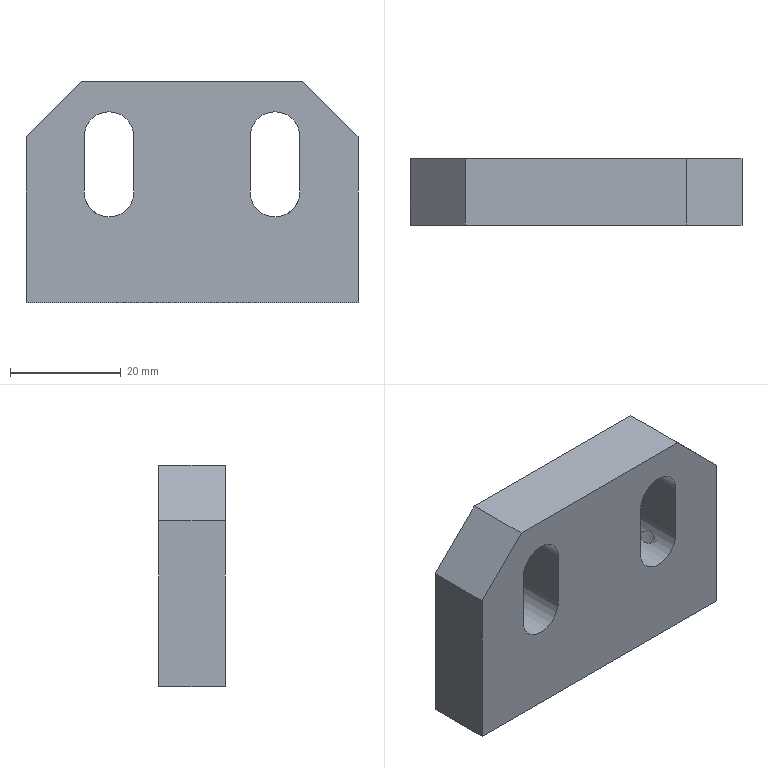Part | SolidWorks | features BaseBody 1 | 1 solid | 30 faces | box 60 x 12 x 40 mm | volume 22885 mm3 | cylinder 12 | plane 12 | cone 6 | commonest cylinder face diameters 5 x6 9 x6
STEP:
#1=CARTESIAN_POINT('',(15.,0.,14.5));
#2=VERTEX_POINT('',#1);
#3=CARTESIAN_POINT('',(19.5,0.,10.));
#4=VERTEX_POINT('',#3);
#5=CARTESIAN_POINT('',(15.,0.,10.));
#6=DIRECTION('',(0.,1.,0.));
#7=DIRECTION('',(0.,0.,-1.));
#8=AXIS2_PLACEMENT_3D('',#5,#6,#7);
#9=CIRCLE('',#8,4.5);
#10=EDGE_CURVE('',#2,#4,#9,.T.);
#11=ORIENTED_EDGE('',*,*,#10,.F.);
#12=CARTESIAN_POINT('',(15.,12.,14.5));
#13=VERTEX_POINT('',#12);
#14=CARTESIAN_POINT('',(15.,0.,14.5));
#15=DIRECTION('',(0.,1.,0.));
#16=VECTOR('',#15,1000.);
#17=LINE('',#14,#16);
#18=EDGE_CURVE('',#2,#13,#17,.T.);
#19=ORIENTED_EDGE('',*,*,#18,.T.);
#20=CARTESIAN_POINT('',(19.5,12.,10.));
#21=VERTEX_POINT('',#20);
#22=CARTESIAN_POINT('',(15.,12.,10.));
#23=DIRECTION('',(0.,1.,0.));
#24=DIRECTION('',(0.,0.,-1.));
#25=AXIS2_PLACEMENT_3D('',#22,#23,#24);
#26=CIRCLE('',#25,4.5);
#27=EDGE_CURVE('',#13,#21,#26,.T.);
#28=ORIENTED_EDGE('',*,*,#27,.T.);
#29=CARTESIAN_POINT('',(19.5,0.,10.));
#30=DIRECTION('',(0.,1.,0.));
#31=VECTOR('',#30,1000.);
#32=LINE('',#29,#31);
#33=EDGE_CURVE('',#4,#21,#32,.T.);
#34=ORIENTED_EDGE('',*,*,#33,.F.);
#35=EDGE_LOOP('',(#11,#19,#28,#34));
#36=FACE_OUTER_BOUND('',#35,.T.);
#37=CARTESIAN_POINT('',(15.,0.,10.));
#38=DIRECTION('',(0.,1.,0.));
#39=DIRECTION('',(0.,0.,1.));
#40=AXIS2_PLACEMENT_3D('',#37,#38,#39);
#41=CYLINDRICAL_SURFACE('',#40,4.5);
#42=ADVANCED_FACE('',(#36),#41,.F.);
#43=CARTESIAN_POINT('',(-15.,0.,14.5));
#44=VERTEX_POINT('',#43);
#45=CARTESIAN_POINT('',(-10.5,0.,10.));
#46=VERTEX_POINT('',#45);
#47=CARTESIAN_POINT('',(-15.,0.,10.));
#48=DIRECTION('',(0.,1.,0.));
#49=DIRECTION('',(0.,0.,1.));
#50=AXIS2_PLACEMENT_3D('',#47,#48,#49);
#51=CIRCLE('',#50,4.5);
#52=EDGE_CURVE('',#44,#46,#51,.T.);
#53=ORIENTED_EDGE('',*,*,#52,.F.);
#54=CARTESIAN_POINT('',(-15.,12.,14.5));
#55=VERTEX_POINT('',#54);
#56=CARTESIAN_POINT('',(-15.,0.,14.5));
#57=DIRECTION('',(0.,1.,0.));
#58=VECTOR('',#57,1000.);
#59=LINE('',#56,#58);
#60=EDGE_CURVE('',#44,#55,#59,.T.);
#61=ORIENTED_EDGE('',*,*,#60,.T.);
#62=CARTESIAN_POINT('',(-10.5,12.,10.));
#63=VERTEX_POINT('',#62);
#64=CARTESIAN_POINT('',(-15.,12.,10.));
#65=DIRECTION('',(0.,1.,0.));
#66=DIRECTION('',(0.,0.,1.));
#67=AXIS2_PLACEMENT_3D('',#64,#65,#66);
#68=CIRCLE('',#67,4.5);
#69=EDGE_CURVE('',#55,#63,#68,.T.);
#70=ORIENTED_EDGE('',*,*,#69,.T.);
#71=CARTESIAN_POINT('',(-10.5,0.,10.));
#72=DIRECTION('',(0.,1.,0.));
#73=VECTOR('',#72,1000.);
#74=LINE('',#71,#73);
#75=EDGE_CURVE('',#46,#63,#74,.T.);
#76=ORIENTED_EDGE('',*,*,#75,.F.);
#77=EDGE_LOOP('',(#53,#61,#70,#76));
#78=FACE_OUTER_BOUND('',#77,.T.);
#79=CARTESIAN_POINT('',(-15.,0.,10.));
#80=DIRECTION('',(0.,1.,0.));
#81=DIRECTION('',(0.,0.,1.));
#82=AXIS2_PLACEMENT_3D('',#79,#80,#81);
#83=CYLINDRICAL_SURFACE('',#82,4.5);
#84=ADVANCED_FACE('',(#78),#83,.F.);
#85=CARTESIAN_POINT('',(22.5,6.,-3.));
#86=VERTEX_POINT('',#85);
#87=CARTESIAN_POINT('',(18.354,4.118,-3.));
#88=VERTEX_POINT('',#87);
#89=CARTESIAN_POINT('',(20.,6.,-3.));
#90=DIRECTION('',(0.,0.,-1.));
#91=DIRECTION('',(-1.,0.,0.));
#92=AXIS2_PLACEMENT_3D('',#89,#90,#91);
#93=CIRCLE('',#92,2.5);
#94=EDGE_CURVE('',#86,#88,#93,.T.);
#95=ORIENTED_EDGE('',*,*,#94,.F.);
#96=CARTESIAN_POINT('',(22.5,6.,-20.));
#97=VERTEX_POINT('',#96);
#98=CARTESIAN_POINT('',(22.5,6.,-20.));
#99=DIRECTION('',(0.,0.,-1.));
#100=VECTOR('',#99,1000.);
#101=LINE('',#98,#100);
#102=EDGE_CURVE('',#86,#97,#101,.T.);
#103=ORIENTED_EDGE('',*,*,#102,.T.);
#104=CARTESIAN_POINT('',(17.5,6.,-20.));
#105=VERTEX_POINT('',#104);
#106=CARTESIAN_POINT('',(20.,6.,-20.));
#107=DIRECTION('',(0.,0.,-1.));
#108=DIRECTION('',(-1.,0.,0.));
#109=AXIS2_PLACEMENT_3D('',#106,#107,#108);
#110=CIRCLE('',#109,2.5);
#111=EDGE_CURVE('',#97,#105,#110,.T.);
#112=ORIENTED_EDGE('',*,*,#111,.T.);
#113=CARTESIAN_POINT('',(17.5,6.,-3.742));
#114=VERTEX_POINT('',#113);
#115=CARTESIAN_POINT('',(17.5,6.,-20.));
#116=DIRECTION('',(0.,0.,-1.));
#117=VECTOR('',#116,1000.);
#118=LINE('',#115,#117);
#119=EDGE_CURVE('',#114,#105,#118,.T.);
#120=ORIENTED_EDGE('',*,*,#119,.F.);
#121=CARTESIAN_POINT('',(17.5,6.,-3.742));
#122=CARTESIAN_POINT('',(17.5,5.807,-3.742));
#123=CARTESIAN_POINT('',(17.522,5.618,-3.727));
#124=CARTESIAN_POINT('',(17.608,5.247,-3.667));
#125=CARTESIAN_POINT('',(17.672,5.071,-3.622));
#126=CARTESIAN_POINT('',(17.83,4.745,-3.5));
#127=CARTESIAN_POINT('',(17.926,4.594,-3.421));
#128=CARTESIAN_POINT('',(18.131,4.331,-3.235));
#129=CARTESIAN_POINT('',(18.243,4.216,-3.125));
#130=CARTESIAN_POINT('',(18.354,4.118,-3.));
#131=B_SPLINE_CURVE_WITH_KNOTS('',3,(#121,#122,#123,#124,#125,#126,#127,#128,#129,#130),.UNSPECIFIED.,.F.,.F.,(4,2,2,2,4),(0.002293,0.002866,0.003438,0.00401,0.004583),.UNSPECIFIED.);
#132=EDGE_CURVE('',#114,#88,#131,.T.);
#133=ORIENTED_EDGE('',*,*,#132,.T.);
#134=EDGE_LOOP('',(#95,#103,#112,#120,#133));
#135=FACE_OUTER_BOUND('',#134,.T.);
#136=CARTESIAN_POINT('',(20.,6.,-20.));
#137=DIRECTION('',(0.,0.,-1.));
#138=DIRECTION('',(-1.,0.,0.));
#139=AXIS2_PLACEMENT_3D('',#136,#137,#138);
#140=CYLINDRICAL_SURFACE('',#139,2.5);
#141=ADVANCED_FACE('',(#135),#140,.F.);
#142=CARTESIAN_POINT('',(20.,6.,-1.498));
#143=VERTEX_POINT('',#142);
#144=CARTESIAN_POINT('',(18.972,6.,-2.116));
#145=VERTEX_POINT('',#144);
#146=CARTESIAN_POINT('',(17.5,6.,-3.));
#147=DIRECTION('',(-0.8572,0.,-0.515));
#148=VECTOR('',#147,1000.);
#149=LINE('',#146,#148);
#150=EDGE_CURVE('',#143,#145,#149,.T.);
#151=ORIENTED_EDGE('',*,*,#150,.F.);
#152=CARTESIAN_POINT('',(22.5,6.,-3.));
#153=DIRECTION('',(0.8572,0.,-0.515));
#154=VECTOR('',#153,1000.);
#155=LINE('',#152,#154);
#156=EDGE_CURVE('',#143,#86,#155,.T.);
#157=ORIENTED_EDGE('',*,*,#156,.T.);
#158=ORIENTED_EDGE('',*,*,#94,.T.);
#159=CARTESIAN_POINT('',(18.354,4.118,-3.));
#160=CARTESIAN_POINT('',(18.522,4.387,-2.812));
#161=CARTESIAN_POINT('',(18.659,4.672,-2.627));
#162=CARTESIAN_POINT('',(18.825,5.136,-2.373));
#163=CARTESIAN_POINT('',(18.873,5.296,-2.292));
#164=CARTESIAN_POINT('',(18.947,5.633,-2.163));
#165=CARTESIAN_POINT('',(18.972,5.814,-2.116));
#166=CARTESIAN_POINT('',(18.972,6.,-2.116));
#167=B_SPLINE_CURVE_WITH_KNOTS('',3,(#159,#160,#161,#162,#163,#164,#165,#166),.UNSPECIFIED.,.F.,.F.,(4,2,2,4),(0.0002918,0.001392,0.001943,0.002493),.UNSPECIFIED.);
#168=EDGE_CURVE('',#88,#145,#167,.T.);
#169=ORIENTED_EDGE('',*,*,#168,.T.);
#170=EDGE_LOOP('',(#151,#157,#158,#169));
#171=FACE_OUTER_BOUND('',#170,.T.);
#172=CARTESIAN_POINT('',(20.,6.,-3.));
#173=DIRECTION('',(0.,0.,-1.));
#174=DIRECTION('',(-1.,0.,0.));
#175=AXIS2_PLACEMENT_3D('',#172,#173,#174);
#176=CONICAL_SURFACE('',#175,2.5,1.03);
#177=ADVANCED_FACE('',(#171),#176,.F.);
#178=CARTESIAN_POINT('',(2.5,6.,-3.));
#179=VERTEX_POINT('',#178);
#180=CARTESIAN_POINT('',(-2.5,6.,-3.));
#181=VERTEX_POINT('',#180);
#182=CARTESIAN_POINT('',(0.,6.,-3.));
#183=DIRECTION('',(0.,0.,-1.));
#184=DIRECTION('',(-1.,0.,0.));
#185=AXIS2_PLACEMENT_3D('',#182,#183,#184);
#186=CIRCLE('',#185,2.5);
#187=EDGE_CURVE('',#179,#181,#186,.T.);
#188=ORIENTED_EDGE('',*,*,#187,.F.);
#189=CARTESIAN_POINT('',(2.5,6.,-20.));
#190=VERTEX_POINT('',#189);
#191=CARTESIAN_POINT('',(2.5,6.,-20.));
#192=DIRECTION('',(0.,0.,-1.));
#193=VECTOR('',#192,1000.);
#194=LINE('',#191,#193);
#195=EDGE_CURVE('',#179,#190,#194,.T.);
#196=ORIENTED_EDGE('',*,*,#195,.T.);
#197=CARTESIAN_POINT('',(-2.5,6.,-20.));
#198=VERTEX_POINT('',#197);
#199=CARTESIAN_POINT('',(0.,6.,-20.));
#200=DIRECTION('',(0.,0.,-1.));
#201=DIRECTION('',(-1.,0.,0.));
#202=AXIS2_PLACEMENT_3D('',#199,#200,#201);
#203=CIRCLE('',#202,2.5);
#204=EDGE_CURVE('',#190,#198,#203,.T.);
#205=ORIENTED_EDGE('',*,*,#204,.T.);
#206=CARTESIAN_POINT('',(-2.5,6.,-20.));
#207=DIRECTION('',(0.,0.,-1.));
#208=VECTOR('',#207,1000.);
#209=LINE('',#206,#208);
#210=EDGE_CURVE('',#181,#198,#209,.T.);
#211=ORIENTED_EDGE('',*,*,#210,.F.);
#212=EDGE_LOOP('',(#188,#196,#205,#211));
#213=FACE_OUTER_BOUND('',#212,.T.);
#214=CARTESIAN_POINT('',(0.,6.,-20.));
#215=DIRECTION('',(0.,0.,-1.));
#216=DIRECTION('',(-1.,0.,0.));
#217=AXIS2_PLACEMENT_3D('',#214,#215,#216);
#218=CYLINDRICAL_SURFACE('',#217,2.5);
#219=ADVANCED_FACE('',(#213),#218,.F.);
#220=CARTESIAN_POINT('',(0.,6.,-1.498));
#221=VERTEX_POINT('',#220);
#222=CARTESIAN_POINT('',(-2.5,6.,-3.));
#223=DIRECTION('',(-0.8572,0.,-0.515));
#224=VECTOR('',#223,1000.);
#225=LINE('',#222,#224);
#226=EDGE_CURVE('',#221,#181,#225,.T.);
#227=ORIENTED_EDGE('',*,*,#226,.F.);
#228=CARTESIAN_POINT('',(2.5,6.,-3.));
#229=DIRECTION('',(0.8572,0.,-0.515));
#230=VECTOR('',#229,1000.);
#231=LINE('',#228,#230);
#232=EDGE_CURVE('',#221,#179,#231,.T.);
#233=ORIENTED_EDGE('',*,*,#232,.T.);
#234=ORIENTED_EDGE('',*,*,#187,.T.);
#235=EDGE_LOOP('',(#227,#233,#234));
#236=FACE_OUTER_BOUND('',#235,.T.);
#237=CARTESIAN_POINT('',(0.,6.,-3.));
#238=DIRECTION('',(0.,0.,-1.));
#239=DIRECTION('',(-1.,0.,0.));
#240=AXIS2_PLACEMENT_3D('',#237,#238,#239);
#241=CONICAL_SURFACE('',#240,2.5,1.03);
#242=ADVANCED_FACE('',(#236),#241,.F.);
#243=CARTESIAN_POINT('',(-18.354,4.118,-3.));
#244=VERTEX_POINT('',#243);
#245=CARTESIAN_POINT('',(-17.5,6.,-3.742));
#246=VERTEX_POINT('',#245);
#247=CARTESIAN_POINT('',(-18.354,4.118,-3.));
#248=CARTESIAN_POINT('',(-18.243,4.216,-3.125));
#249=CARTESIAN_POINT('',(-18.133,4.329,-3.233));
#250=CARTESIAN_POINT('',(-17.927,4.593,-3.421));
#251=CARTESIAN_POINT('',(-17.831,4.743,-3.499));
#252=CARTESIAN_POINT('',(-17.673,5.068,-3.621));
#253=CARTESIAN_POINT('',(-17.609,5.247,-3.667));
#254=CARTESIAN_POINT('',(-17.522,5.616,-3.727));
#255=CARTESIAN_POINT('',(-17.5,5.807,-3.742));
#256=CARTESIAN_POINT('',(-17.5,6.,-3.742));
#257=B_SPLINE_CURVE_WITH_KNOTS('',3,(#247,#248,#249,#250,#251,#252,#253,#254,#255,#256),.UNSPECIFIED.,.F.,.F.,(4,2,2,2,4),(0.,0.0005733,0.001147,0.00172,0.002293),.UNSPECIFIED.);
#258=EDGE_CURVE('',#244,#246,#257,.T.);
#259=ORIENTED_EDGE('',*,*,#258,.T.);
#260=CARTESIAN_POINT('',(-17.5,6.,-20.));
#261=VERTEX_POINT('',#260);
#262=CARTESIAN_POINT('',(-17.5,6.,-20.));
#263=DIRECTION('',(0.,0.,-1.));
#264=VECTOR('',#263,1000.);
#265=LINE('',#262,#264);
#266=EDGE_CURVE('',#246,#261,#265,.T.);
#267=ORIENTED_EDGE('',*,*,#266,.T.);
#268=CARTESIAN_POINT('',(-22.5,6.,-20.));
#269=VERTEX_POINT('',#268);
#270=CARTESIAN_POINT('',(-20.,6.,-20.));
#271=DIRECTION('',(0.,0.,-1.));
#272=DIRECTION('',(-1.,0.,0.));
#273=AXIS2_PLACEMENT_3D('',#270,#271,#272);
#274=CIRCLE('',#273,2.5);
#275=EDGE_CURVE('',#261,#269,#274,.T.);
#276=ORIENTED_EDGE('',*,*,#275,.T.);
#277=CARTESIAN_POINT('',(-22.5,6.,-3.));
#278=VERTEX_POINT('',#277);
#279=CARTESIAN_POINT('',(-22.5,6.,-20.));
#280=DIRECTION('',(0.,0.,-1.));
#281=VECTOR('',#280,1000.);
#282=LINE('',#279,#281);
#283=EDGE_CURVE('',#278,#269,#282,.T.);
#284=ORIENTED_EDGE('',*,*,#283,.F.);
#285=CARTESIAN_POINT('',(-20.,6.,-3.));
#286=DIRECTION('',(0.,0.,-1.));
#287=DIRECTION('',(-1.,0.,0.));
#288=AXIS2_PLACEMENT_3D('',#285,#286,#287);
#289=CIRCLE('',#288,2.5);
#290=EDGE_CURVE('',#244,#278,#289,.T.);
#291=ORIENTED_EDGE('',*,*,#290,.F.);
#292=EDGE_LOOP('',(#259,#267,#276,#284,#291));
#293=FACE_OUTER_BOUND('',#292,.T.);
#294=CARTESIAN_POINT('',(-20.,6.,-20.));
#295=DIRECTION('',(0.,0.,-1.));
#296=DIRECTION('',(-1.,0.,0.));
#297=AXIS2_PLACEMENT_3D('',#294,#295,#296);
#298=CYLINDRICAL_SURFACE('',#297,2.5);
#299=ADVANCED_FACE('',(#293),#298,.F.);
#300=CARTESIAN_POINT('',(-20.,6.,-1.498));
#301=VERTEX_POINT('',#300);
#302=CARTESIAN_POINT('',(-22.5,6.,-3.));
#303=DIRECTION('',(-0.8572,0.,-0.515));
#304=VECTOR('',#303,1000.);
#305=LINE('',#302,#304);
#306=EDGE_CURVE('',#301,#278,#305,.T.);
#307=ORIENTED_EDGE('',*,*,#306,.F.);
#308=CARTESIAN_POINT('',(-18.972,6.,-2.116));
#309=VERTEX_POINT('',#308);
#310=CARTESIAN_POINT('',(-17.5,6.,-3.));
#311=DIRECTION('',(0.8572,0.,-0.515));
#312=VECTOR('',#311,1000.);
#313=LINE('',#310,#312);
#314=EDGE_CURVE('',#301,#309,#313,.T.);
#315=ORIENTED_EDGE('',*,*,#314,.T.);
#316=CARTESIAN_POINT('',(-18.972,6.,-2.116));
#317=CARTESIAN_POINT('',(-18.972,5.813,-2.116));
#318=CARTESIAN_POINT('',(-18.947,5.632,-2.163));
#319=CARTESIAN_POINT('',(-18.873,5.294,-2.293));
#320=CARTESIAN_POINT('',(-18.825,5.136,-2.373));
#321=CARTESIAN_POINT('',(-18.715,4.829,-2.541));
#322=CARTESIAN_POINT('',(-18.653,4.68,-2.631));
#323=CARTESIAN_POINT('',(-18.514,4.392,-2.813));
#324=CARTESIAN_POINT('',(-18.438,4.252,-2.906));
#325=CARTESIAN_POINT('',(-18.354,4.118,-3.));
#326=B_SPLINE_CURVE_WITH_KNOTS('',3,(#316,#317,#318,#319,#320,#321,#322,#323,#324,#325),.UNSPECIFIED.,.F.,.F.,(4,2,2,2,4),(0.002493,0.003044,0.003596,0.004147,0.004698),.UNSPECIFIED.);
#327=EDGE_CURVE('',#309,#244,#326,.T.);
#328=ORIENTED_EDGE('',*,*,#327,.T.);
#329=ORIENTED_EDGE('',*,*,#290,.T.);
#330=EDGE_LOOP('',(#307,#315,#328,#329));
#331=FACE_OUTER_BOUND('',#330,.T.);
#332=CARTESIAN_POINT('',(-20.,6.,-3.));
#333=DIRECTION('',(0.,0.,-1.));
#334=DIRECTION('',(-1.,0.,0.));
#335=AXIS2_PLACEMENT_3D('',#332,#333,#334);
#336=CONICAL_SURFACE('',#335,2.5,1.03);
#337=ADVANCED_FACE('',(#331),#336,.F.);
#338=CARTESIAN_POINT('',(-30.,0.,-20.));
#339=VERTEX_POINT('',#338);
#340=CARTESIAN_POINT('',(-30.,0.,10.));
#341=VERTEX_POINT('',#340);
#342=CARTESIAN_POINT('',(-30.,0.,-20.));
#343=DIRECTION('',(0.,0.,1.));
#344=VECTOR('',#343,1000.);
#345=LINE('',#342,#344);
#346=EDGE_CURVE('',#339,#341,#345,.T.);
#347=ORIENTED_EDGE('',*,*,#346,.T.);
#348=CARTESIAN_POINT('',(-30.,12.,10.));
#349=VERTEX_POINT('',#348);
#350=CARTESIAN_POINT('',(-30.,12.,10.));
#351=DIRECTION('',(0.,1.,0.));
#352=VECTOR('',#351,1000.);
#353=LINE('',#350,#352);
#354=EDGE_CURVE('',#341,#349,#353,.T.);
#355=ORIENTED_EDGE('',*,*,#354,.T.);
#356=CARTESIAN_POINT('',(-30.,12.,-20.));
#357=VERTEX_POINT('',#356);
#358=CARTESIAN_POINT('',(-30.,12.,-20.));
#359=DIRECTION('',(0.,0.,1.));
#360=VECTOR('',#359,1000.);
#361=LINE('',#358,#360);
#362=EDGE_CURVE('',#357,#349,#361,.T.);
#363=ORIENTED_EDGE('',*,*,#362,.F.);
#364=CARTESIAN_POINT('',(-30.,12.,-20.));
#365=DIRECTION('',(0.,-1.,0.));
#366=VECTOR('',#365,1000.);
#367=LINE('',#364,#366);
#368=EDGE_CURVE('',#357,#339,#367,.T.);
#369=ORIENTED_EDGE('',*,*,#368,.T.);
#370=EDGE_LOOP('',(#347,#355,#363,#369));
#371=FACE_OUTER_BOUND('',#370,.T.);
#372=CARTESIAN_POINT('',(-30.,12.,-20.));
#373=DIRECTION('',(1.,0.,0.));
#374=DIRECTION('',(0.,0.,-1.));
#375=AXIS2_PLACEMENT_3D('',#372,#373,#374);
#376=PLANE('',#375);
#377=ADVANCED_FACE('',(#371),#376,.F.);
#378=CARTESIAN_POINT('',(-20.,0.,20.));
#379=VERTEX_POINT('',#378);
#380=CARTESIAN_POINT('',(20.,0.,20.));
#381=VERTEX_POINT('',#380);
#382=CARTESIAN_POINT('',(30.,0.,20.));
#383=DIRECTION('',(1.,0.,0.));
#384=VECTOR('',#383,1000.);
#385=LINE('',#382,#384);
#386=EDGE_CURVE('',#379,#381,#385,.T.);
#387=ORIENTED_EDGE('',*,*,#386,.T.);
#388=CARTESIAN_POINT('',(20.,12.,20.));
#389=VERTEX_POINT('',#388);
#390=CARTESIAN_POINT('',(20.,12.,20.));
#391=DIRECTION('',(0.,1.,0.));
#392=VECTOR('',#391,1000.);
#393=LINE('',#390,#392);
#394=EDGE_CURVE('',#381,#389,#393,.T.);
#395=ORIENTED_EDGE('',*,*,#394,.T.);
#396=CARTESIAN_POINT('',(-20.,12.,20.));
#397=VERTEX_POINT('',#396);
#398=CARTESIAN_POINT('',(30.,12.,20.));
#399=DIRECTION('',(1.,0.,0.));
#400=VECTOR('',#399,1000.);
#401=LINE('',#398,#400);
#402=EDGE_CURVE('',#397,#389,#401,.T.);
#403=ORIENTED_EDGE('',*,*,#402,.F.);
#404=CARTESIAN_POINT('',(-20.,12.,20.));
#405=DIRECTION('',(0.,-1.,0.));
#406=VECTOR('',#405,1000.);
#407=LINE('',#404,#406);
#408=EDGE_CURVE('',#397,#379,#407,.T.);
#409=ORIENTED_EDGE('',*,*,#408,.T.);
#410=EDGE_LOOP('',(#387,#395,#403,#409));
#411=FACE_OUTER_BOUND('',#410,.T.);
#412=CARTESIAN_POINT('',(30.,12.,20.));
#413=DIRECTION('',(0.,0.,-1.));
#414=DIRECTION('',(-1.,0.,0.));
#415=AXIS2_PLACEMENT_3D('',#412,#413,#414);
#416=PLANE('',#415);
#417=ADVANCED_FACE('',(#411),#416,.F.);
#418=CARTESIAN_POINT('',(30.,12.,10.));
#419=VERTEX_POINT('',#418);
#420=CARTESIAN_POINT('',(30.,12.,-20.));
#421=VERTEX_POINT('',#420);
#422=CARTESIAN_POINT('',(30.,12.,-20.));
#423=DIRECTION('',(0.,0.,-1.));
#424=VECTOR('',#423,1000.);
#425=LINE('',#422,#424);
#426=EDGE_CURVE('',#419,#421,#425,.T.);
#427=ORIENTED_EDGE('',*,*,#426,.F.);
#428=CARTESIAN_POINT('',(30.,0.,10.));
#429=VERTEX_POINT('',#428);
#430=CARTESIAN_POINT('',(30.,12.,10.));
#431=DIRECTION('',(0.,-1.,0.));
#432=VECTOR('',#431,1000.);
#433=LINE('',#430,#432);
#434=EDGE_CURVE('',#419,#429,#433,.T.);
#435=ORIENTED_EDGE('',*,*,#434,.T.);
#436=CARTESIAN_POINT('',(30.,0.,-20.));
#437=VERTEX_POINT('',#436);
#438=CARTESIAN_POINT('',(30.,0.,-20.));
#439=DIRECTION('',(0.,0.,-1.));
#440=VECTOR('',#439,1000.);
#441=LINE('',#438,#440);
#442=EDGE_CURVE('',#429,#437,#441,.T.);
#443=ORIENTED_EDGE('',*,*,#442,.T.);
#444=CARTESIAN_POINT('',(30.,12.,-20.));
#445=DIRECTION('',(0.,-1.,0.));
#446=VECTOR('',#445,1000.);
#447=LINE('',#444,#446);
#448=EDGE_CURVE('',#421,#437,#447,.T.);
#449=ORIENTED_EDGE('',*,*,#448,.F.);
#450=EDGE_LOOP('',(#427,#435,#443,#449));
#451=FACE_OUTER_BOUND('',#450,.T.);
#452=CARTESIAN_POINT('',(30.,12.,-20.));
#453=DIRECTION('',(-1.,0.,0.));
#454=DIRECTION('',(0.,0.,1.));
#455=AXIS2_PLACEMENT_3D('',#452,#453,#454);
#456=PLANE('',#455);
#457=ADVANCED_FACE('',(#451),#456,.F.);
#458=CARTESIAN_POINT('',(20.,6.,-20.));
#459=DIRECTION('',(0.,0.,-1.));
#460=DIRECTION('',(-1.,0.,0.));
#461=AXIS2_PLACEMENT_3D('',#458,#459,#460);
#462=CIRCLE('',#461,2.5);
#463=EDGE_CURVE('',#105,#97,#462,.T.);
#464=ORIENTED_EDGE('',*,*,#463,.F.);
#465=ORIENTED_EDGE('',*,*,#111,.F.);
#466=EDGE_LOOP('',(#464,#465));
#467=FACE_BOUND('',#466,.T.);
#468=CARTESIAN_POINT('',(0.,6.,-20.));
#469=DIRECTION('',(0.,0.,-1.));
#470=DIRECTION('',(-1.,0.,0.));
#471=AXIS2_PLACEMENT_3D('',#468,#469,#470);
#472=CIRCLE('',#471,2.5);
#473=EDGE_CURVE('',#198,#190,#472,.T.);
#474=ORIENTED_EDGE('',*,*,#473,.F.);
#475=ORIENTED_EDGE('',*,*,#204,.F.);
#476=EDGE_LOOP('',(#474,#475));
#477=FACE_BOUND('',#476,.T.);
#478=CARTESIAN_POINT('',(-20.,6.,-20.));
#479=DIRECTION('',(0.,0.,-1.));
#480=DIRECTION('',(-1.,0.,0.));
#481=AXIS2_PLACEMENT_3D('',#478,#479,#480);
#482=CIRCLE('',#481,2.5);
#483=EDGE_CURVE('',#269,#261,#482,.T.);
#484=ORIENTED_EDGE('',*,*,#483,.F.);
#485=ORIENTED_EDGE('',*,*,#275,.F.);
#486=EDGE_LOOP('',(#484,#485));
#487=FACE_BOUND('',#486,.T.);
#488=CARTESIAN_POINT('',(30.,0.,-20.));
#489=DIRECTION('',(-1.,0.,0.));
#490=VECTOR('',#489,1000.);
#491=LINE('',#488,#490);
#492=EDGE_CURVE('',#437,#339,#491,.T.);
#493=ORIENTED_EDGE('',*,*,#492,.T.);
#494=ORIENTED_EDGE('',*,*,#368,.F.);
#495=CARTESIAN_POINT('',(30.,12.,-20.));
#496=DIRECTION('',(-1.,0.,0.));
#497=VECTOR('',#496,1000.);
#498=LINE('',#495,#497);
#499=EDGE_CURVE('',#421,#357,#498,.T.);
#500=ORIENTED_EDGE('',*,*,#499,.F.);
#501=ORIENTED_EDGE('',*,*,#448,.T.);
#502=EDGE_LOOP('',(#493,#494,#500,#501));
#503=FACE_OUTER_BOUND('',#502,.T.);
#504=CARTESIAN_POINT('',(30.,12.,-20.));
#505=DIRECTION('',(0.,0.,1.));
#506=DIRECTION('',(1.,0.,0.));
#507=AXIS2_PLACEMENT_3D('',#504,#505,#506);
#508=PLANE('',#507);
#509=ADVANCED_FACE('',(#467,#477,#487,#503),#508,.F.);
#510=CARTESIAN_POINT('',(10.5,12.,0.));
#511=VERTEX_POINT('',#510);
#512=CARTESIAN_POINT('',(10.5,12.,10.));
#513=VERTEX_POINT('',#512);
#514=CARTESIAN_POINT('',(10.5,12.,0.));
#515=DIRECTION('',(0.,0.,1.));
#516=VECTOR('',#515,1000.);
#517=LINE('',#514,#516);
#518=EDGE_CURVE('',#511,#513,#517,.T.);
#519=ORIENTED_EDGE('',*,*,#518,.F.);
#520=CARTESIAN_POINT('',(19.5,12.,0.));
#521=VERTEX_POINT('',#520);
#522=CARTESIAN_POINT('',(15.,12.,0.));
#523=DIRECTION('',(0.,1.,0.));
#524=DIRECTION('',(0.,0.,-1.));
#525=AXIS2_PLACEMENT_3D('',#522,#523,#524);
#526=CIRCLE('',#525,4.5);
#527=EDGE_CURVE('',#521,#511,#526,.T.);
#528=ORIENTED_EDGE('',*,*,#527,.F.);
#529=CARTESIAN_POINT('',(19.5,12.,0.));
#530=DIRECTION('',(0.,0.,-1.));
#531=VECTOR('',#530,1000.);
#532=LINE('',#529,#531);
#533=EDGE_CURVE('',#21,#521,#532,.T.);
#534=ORIENTED_EDGE('',*,*,#533,.F.);
#535=ORIENTED_EDGE('',*,*,#27,.F.);
#536=CARTESIAN_POINT('',(15.,12.,10.));
#537=DIRECTION('',(0.,1.,0.));
#538=DIRECTION('',(0.,0.,-1.));
#539=AXIS2_PLACEMENT_3D('',#536,#537,#538);
#540=CIRCLE('',#539,4.5);
#541=EDGE_CURVE('',#513,#13,#540,.T.);
#542=ORIENTED_EDGE('',*,*,#541,.F.);
#543=EDGE_LOOP('',(#519,#528,#534,#535,#542));
#544=FACE_BOUND('',#543,.T.);
#545=CARTESIAN_POINT('',(-19.5,12.,0.));
#546=VERTEX_POINT('',#545);
#547=CARTESIAN_POINT('',(-19.5,12.,10.));
#548=VERTEX_POINT('',#547);
#549=CARTESIAN_POINT('',(-19.5,12.,0.));
#550=DIRECTION('',(0.,0.,1.));
#551=VECTOR('',#550,1000.);
#552=LINE('',#549,#551);
#553=EDGE_CURVE('',#546,#548,#552,.T.);
#554=ORIENTED_EDGE('',*,*,#553,.F.);
#555=CARTESIAN_POINT('',(-10.5,12.,0.));
#556=VERTEX_POINT('',#555);
#557=CARTESIAN_POINT('',(-15.,12.,0.));
#558=DIRECTION('',(0.,1.,0.));
#559=DIRECTION('',(0.,0.,1.));
#560=AXIS2_PLACEMENT_3D('',#557,#558,#559);
#561=CIRCLE('',#560,4.5);
#562=EDGE_CURVE('',#556,#546,#561,.T.);
#563=ORIENTED_EDGE('',*,*,#562,.F.);
#564=CARTESIAN_POINT('',(-10.5,12.,0.));
#565=DIRECTION('',(0.,0.,-1.));
#566=VECTOR('',#565,1000.);
#567=LINE('',#564,#566);
#568=EDGE_CURVE('',#63,#556,#567,.T.);
#569=ORIENTED_EDGE('',*,*,#568,.F.);
#570=ORIENTED_EDGE('',*,*,#69,.F.);
#571=CARTESIAN_POINT('',(-15.,12.,10.));
#572=DIRECTION('',(0.,1.,0.));
#573=DIRECTION('',(0.,0.,1.));
#574=AXIS2_PLACEMENT_3D('',#571,#572,#573);
#575=CIRCLE('',#574,4.5);
#576=EDGE_CURVE('',#548,#55,#575,.T.);
#577=ORIENTED_EDGE('',*,*,#576,.F.);
#578=EDGE_LOOP('',(#554,#563,#569,#570,#577));
#579=FACE_BOUND('',#578,.T.);
#580=ORIENTED_EDGE('',*,*,#402,.T.);
#581=CARTESIAN_POINT('',(30.,12.,10.));
#582=DIRECTION('',(0.7071,0.,-0.7071));
#583=VECTOR('',#582,1000.);
#584=LINE('',#581,#583);
#585=EDGE_CURVE('',#389,#419,#584,.T.);
#586=ORIENTED_EDGE('',*,*,#585,.T.);
#587=ORIENTED_EDGE('',*,*,#426,.T.);
#588=ORIENTED_EDGE('',*,*,#499,.T.);
#589=ORIENTED_EDGE('',*,*,#362,.T.);
#590=CARTESIAN_POINT('',(-20.,12.,20.));
#591=DIRECTION('',(0.7071,0.,0.7071));
#592=VECTOR('',#591,1000.);
#593=LINE('',#590,#592);
#594=EDGE_CURVE('',#349,#397,#593,.T.);
#595=ORIENTED_EDGE('',*,*,#594,.T.);
#596=EDGE_LOOP('',(#580,#586,#587,#588,#589,#595));
#597=FACE_OUTER_BOUND('',#596,.T.);
#598=CARTESIAN_POINT('',(0.,12.,0.));
#599=DIRECTION('',(0.,-1.,0.));
#600=DIRECTION('',(0.,0.,-1.));
#601=AXIS2_PLACEMENT_3D('',#598,#599,#600);
#602=PLANE('',#601);
#603=ADVANCED_FACE('',(#544,#579,#597),#602,.F.);
#604=CARTESIAN_POINT('',(19.5,0.,0.));
#605=VERTEX_POINT('',#604);
#606=CARTESIAN_POINT('',(10.5,0.,0.));
#607=VERTEX_POINT('',#606);
#608=CARTESIAN_POINT('',(15.,0.,0.));
#609=DIRECTION('',(0.,1.,0.));
#610=DIRECTION('',(0.,0.,-1.));
#611=AXIS2_PLACEMENT_3D('',#608,#609,#610);
#612=CIRCLE('',#611,4.5);
#613=EDGE_CURVE('',#605,#607,#612,.T.);
#614=ORIENTED_EDGE('',*,*,#613,.T.);
#615=CARTESIAN_POINT('',(10.5,0.,10.));
#616=VERTEX_POINT('',#615);
#617=CARTESIAN_POINT('',(10.5,0.,0.));
#618=DIRECTION('',(0.,0.,1.));
#619=VECTOR('',#618,1000.);
#620=LINE('',#617,#619);
#621=EDGE_CURVE('',#607,#616,#620,.T.);
#622=ORIENTED_EDGE('',*,*,#621,.T.);
#623=CARTESIAN_POINT('',(15.,0.,10.));
#624=DIRECTION('',(0.,1.,0.));
#625=DIRECTION('',(0.,0.,-1.));
#626=AXIS2_PLACEMENT_3D('',#623,#624,#625);
#627=CIRCLE('',#626,4.5);
#628=EDGE_CURVE('',#616,#2,#627,.T.);
#629=ORIENTED_EDGE('',*,*,#628,.T.);
#630=ORIENTED_EDGE('',*,*,#10,.T.);
#631=CARTESIAN_POINT('',(19.5,0.,0.));
#632=DIRECTION('',(0.,0.,-1.));
#633=VECTOR('',#632,1000.);
#634=LINE('',#631,#633);
#635=EDGE_CURVE('',#4,#605,#634,.T.);
#636=ORIENTED_EDGE('',*,*,#635,.T.);
#637=EDGE_LOOP('',(#614,#622,#629,#630,#636));
#638=FACE_BOUND('',#637,.T.);
#639=CARTESIAN_POINT('',(-10.5,0.,0.));
#640=VERTEX_POINT('',#639);
#641=CARTESIAN_POINT('',(-19.5,0.,0.));
#642=VERTEX_POINT('',#641);
#643=CARTESIAN_POINT('',(-15.,0.,0.));
#644=DIRECTION('',(0.,1.,0.));
#645=DIRECTION('',(0.,0.,1.));
#646=AXIS2_PLACEMENT_3D('',#643,#644,#645);
#647=CIRCLE('',#646,4.5);
#648=EDGE_CURVE('',#640,#642,#647,.T.);
#649=ORIENTED_EDGE('',*,*,#648,.T.);
#650=CARTESIAN_POINT('',(-19.5,0.,10.));
#651=VERTEX_POINT('',#650);
#652=CARTESIAN_POINT('',(-19.5,0.,0.));
#653=DIRECTION('',(0.,0.,1.));
#654=VECTOR('',#653,1000.);
#655=LINE('',#652,#654);
#656=EDGE_CURVE('',#642,#651,#655,.T.);
#657=ORIENTED_EDGE('',*,*,#656,.T.);
#658=CARTESIAN_POINT('',(-15.,0.,10.));
#659=DIRECTION('',(0.,1.,0.));
#660=DIRECTION('',(0.,0.,1.));
#661=AXIS2_PLACEMENT_3D('',#658,#659,#660);
#662=CIRCLE('',#661,4.5);
#663=EDGE_CURVE('',#651,#44,#662,.T.);
#664=ORIENTED_EDGE('',*,*,#663,.T.);
#665=ORIENTED_EDGE('',*,*,#52,.T.);
#666=CARTESIAN_POINT('',(-10.5,0.,0.));
#667=DIRECTION('',(0.,0.,-1.));
#668=VECTOR('',#667,1000.);
#669=LINE('',#666,#668);
#670=EDGE_CURVE('',#46,#640,#669,.T.);
#671=ORIENTED_EDGE('',*,*,#670,.T.);
#672=EDGE_LOOP('',(#649,#657,#664,#665,#671));
#673=FACE_BOUND('',#672,.T.);
#674=ORIENTED_EDGE('',*,*,#442,.F.);
#675=CARTESIAN_POINT('',(20.,0.,20.));
#676=DIRECTION('',(-0.7071,0.,0.7071));
#677=VECTOR('',#676,1000.);
#678=LINE('',#675,#677);
#679=EDGE_CURVE('',#429,#381,#678,.T.);
#680=ORIENTED_EDGE('',*,*,#679,.T.);
#681=ORIENTED_EDGE('',*,*,#386,.F.);
#682=CARTESIAN_POINT('',(-20.,0.,20.));
#683=DIRECTION('',(-0.7071,0.,-0.7071));
#684=VECTOR('',#683,1000.);
#685=LINE('',#682,#684);
#686=EDGE_CURVE('',#379,#341,#685,.T.);
#687=ORIENTED_EDGE('',*,*,#686,.T.);
#688=ORIENTED_EDGE('',*,*,#346,.F.);
#689=ORIENTED_EDGE('',*,*,#492,.F.);
#690=EDGE_LOOP('',(#674,#680,#681,#687,#688,#689));
#691=FACE_OUTER_BOUND('',#690,.T.);
#692=CARTESIAN_POINT('',(0.,0.,0.));
#693=DIRECTION('',(0.,-1.,0.));
#694=DIRECTION('',(0.,0.,-1.));
#695=AXIS2_PLACEMENT_3D('',#692,#693,#694);
#696=PLANE('',#695);
#697=ADVANCED_FACE('',(#638,#673,#691),#696,.T.);
#698=ORIENTED_EDGE('',*,*,#314,.F.);
#699=ORIENTED_EDGE('',*,*,#306,.T.);
#700=CARTESIAN_POINT('',(-18.354,7.882,-3.));
#701=VERTEX_POINT('',#700);
#702=CARTESIAN_POINT('',(-20.,6.,-3.));
#703=DIRECTION('',(0.,0.,-1.));
#704=DIRECTION('',(-1.,0.,0.));
#705=AXIS2_PLACEMENT_3D('',#702,#703,#704);
#706=CIRCLE('',#705,2.5);
#707=EDGE_CURVE('',#278,#701,#706,.T.);
#708=ORIENTED_EDGE('',*,*,#707,.T.);
#709=CARTESIAN_POINT('',(-18.354,7.882,-3.));
#710=CARTESIAN_POINT('',(-18.522,7.613,-2.812));
#711=CARTESIAN_POINT('',(-18.659,7.328,-2.627));
#712=CARTESIAN_POINT('',(-18.825,6.864,-2.373));
#713=CARTESIAN_POINT('',(-18.873,6.704,-2.292));
#714=CARTESIAN_POINT('',(-18.947,6.367,-2.163));
#715=CARTESIAN_POINT('',(-18.972,6.186,-2.116));
#716=CARTESIAN_POINT('',(-18.972,6.,-2.116));
#717=B_SPLINE_CURVE_WITH_KNOTS('',3,(#709,#710,#711,#712,#713,#714,#715,#716),.UNSPECIFIED.,.F.,.F.,(4,2,2,4),(0.0002918,0.001392,0.001943,0.002493),.UNSPECIFIED.);
#718=EDGE_CURVE('',#701,#309,#717,.T.);
#719=ORIENTED_EDGE('',*,*,#718,.T.);
#720=EDGE_LOOP('',(#698,#699,#708,#719));
#721=FACE_OUTER_BOUND('',#720,.T.);
#722=CARTESIAN_POINT('',(-20.,6.,-3.));
#723=DIRECTION('',(0.,0.,-1.));
#724=DIRECTION('',(-1.,0.,0.));
#725=AXIS2_PLACEMENT_3D('',#722,#723,#724);
#726=CONICAL_SURFACE('',#725,2.5,1.03);
#727=ADVANCED_FACE('',(#721),#726,.F.);
#728=ORIENTED_EDGE('',*,*,#266,.F.);
#729=CARTESIAN_POINT('',(-17.5,6.,-3.742));
#730=CARTESIAN_POINT('',(-17.5,6.193,-3.742));
#731=CARTESIAN_POINT('',(-17.522,6.382,-3.727));
#732=CARTESIAN_POINT('',(-17.608,6.753,-3.667));
#733=CARTESIAN_POINT('',(-17.672,6.929,-3.622));
#734=CARTESIAN_POINT('',(-17.83,7.255,-3.5));
#735=CARTESIAN_POINT('',(-17.926,7.406,-3.421));
#736=CARTESIAN_POINT('',(-18.131,7.669,-3.235));
#737=CARTESIAN_POINT('',(-18.243,7.784,-3.125));
#738=CARTESIAN_POINT('',(-18.354,7.882,-3.));
#739=B_SPLINE_CURVE_WITH_KNOTS('',3,(#729,#730,#731,#732,#733,#734,#735,#736,#737,#738),.UNSPECIFIED.,.F.,.F.,(4,2,2,2,4),(0.002293,0.002866,0.003438,0.00401,0.004583),.UNSPECIFIED.);
#740=EDGE_CURVE('',#246,#701,#739,.T.);
#741=ORIENTED_EDGE('',*,*,#740,.T.);
#742=ORIENTED_EDGE('',*,*,#707,.F.);
#743=ORIENTED_EDGE('',*,*,#283,.T.);
#744=ORIENTED_EDGE('',*,*,#483,.T.);
#745=EDGE_LOOP('',(#728,#741,#742,#743,#744));
#746=FACE_OUTER_BOUND('',#745,.T.);
#747=CARTESIAN_POINT('',(-20.,6.,-20.));
#748=DIRECTION('',(0.,0.,-1.));
#749=DIRECTION('',(-1.,0.,0.));
#750=AXIS2_PLACEMENT_3D('',#747,#748,#749);
#751=CYLINDRICAL_SURFACE('',#750,2.5);
#752=ADVANCED_FACE('',(#746),#751,.F.);
#753=ORIENTED_EDGE('',*,*,#232,.F.);
#754=ORIENTED_EDGE('',*,*,#226,.T.);
#755=CARTESIAN_POINT('',(0.,6.,-3.));
#756=DIRECTION('',(0.,0.,-1.));
#757=DIRECTION('',(-1.,0.,0.));
#758=AXIS2_PLACEMENT_3D('',#755,#756,#757);
#759=CIRCLE('',#758,2.5);
#760=EDGE_CURVE('',#181,#179,#759,.T.);
#761=ORIENTED_EDGE('',*,*,#760,.T.);
#762=EDGE_LOOP('',(#753,#754,#761));
#763=FACE_OUTER_BOUND('',#762,.T.);
#764=CARTESIAN_POINT('',(0.,6.,-3.));
#765=DIRECTION('',(0.,0.,-1.));
#766=DIRECTION('',(-1.,0.,0.));
#767=AXIS2_PLACEMENT_3D('',#764,#765,#766);
#768=CONICAL_SURFACE('',#767,2.5,1.03);
#769=ADVANCED_FACE('',(#763),#768,.F.);
#770=ORIENTED_EDGE('',*,*,#195,.F.);
#771=ORIENTED_EDGE('',*,*,#760,.F.);
#772=ORIENTED_EDGE('',*,*,#210,.T.);
#773=ORIENTED_EDGE('',*,*,#473,.T.);
#774=EDGE_LOOP('',(#770,#771,#772,#773));
#775=FACE_OUTER_BOUND('',#774,.T.);
#776=CARTESIAN_POINT('',(0.,6.,-20.));
#777=DIRECTION('',(0.,0.,-1.));
#778=DIRECTION('',(-1.,0.,0.));
#779=AXIS2_PLACEMENT_3D('',#776,#777,#778);
#780=CYLINDRICAL_SURFACE('',#779,2.5);
#781=ADVANCED_FACE('',(#775),#780,.F.);
#782=ORIENTED_EDGE('',*,*,#156,.F.);
#783=ORIENTED_EDGE('',*,*,#150,.T.);
#784=CARTESIAN_POINT('',(18.354,7.882,-3.));
#785=VERTEX_POINT('',#784);
#786=CARTESIAN_POINT('',(18.972,6.,-2.116));
#787=CARTESIAN_POINT('',(18.972,6.187,-2.116));
#788=CARTESIAN_POINT('',(18.947,6.368,-2.163));
#789=CARTESIAN_POINT('',(18.873,6.706,-2.293));
#790=CARTESIAN_POINT('',(18.825,6.864,-2.373));
#791=CARTESIAN_POINT('',(18.715,7.171,-2.541));
#792=CARTESIAN_POINT('',(18.653,7.32,-2.631));
#793=CARTESIAN_POINT('',(18.514,7.608,-2.813));
#794=CARTESIAN_POINT('',(18.438,7.748,-2.906));
#795=CARTESIAN_POINT('',(18.354,7.882,-3.));
#796=B_SPLINE_CURVE_WITH_KNOTS('',3,(#786,#787,#788,#789,#790,#791,#792,#793,#794,#795),.UNSPECIFIED.,.F.,.F.,(4,2,2,2,4),(0.002493,0.003044,0.003596,0.004147,0.004698),.UNSPECIFIED.);
#797=EDGE_CURVE('',#145,#785,#796,.T.);
#798=ORIENTED_EDGE('',*,*,#797,.T.);
#799=CARTESIAN_POINT('',(20.,6.,-3.));
#800=DIRECTION('',(0.,0.,-1.));
#801=DIRECTION('',(-1.,0.,0.));
#802=AXIS2_PLACEMENT_3D('',#799,#800,#801);
#803=CIRCLE('',#802,2.5);
#804=EDGE_CURVE('',#785,#86,#803,.T.);
#805=ORIENTED_EDGE('',*,*,#804,.T.);
#806=EDGE_LOOP('',(#782,#783,#798,#805));
#807=FACE_OUTER_BOUND('',#806,.T.);
#808=CARTESIAN_POINT('',(20.,6.,-3.));
#809=DIRECTION('',(0.,0.,-1.));
#810=DIRECTION('',(-1.,0.,0.));
#811=AXIS2_PLACEMENT_3D('',#808,#809,#810);
#812=CONICAL_SURFACE('',#811,2.5,1.03);
#813=ADVANCED_FACE('',(#807),#812,.F.);
#814=ORIENTED_EDGE('',*,*,#102,.F.);
#815=ORIENTED_EDGE('',*,*,#804,.F.);
#816=CARTESIAN_POINT('',(18.354,7.882,-3.));
#817=CARTESIAN_POINT('',(18.243,7.784,-3.125));
#818=CARTESIAN_POINT('',(18.133,7.671,-3.233));
#819=CARTESIAN_POINT('',(17.927,7.407,-3.421));
#820=CARTESIAN_POINT('',(17.831,7.257,-3.499));
#821=CARTESIAN_POINT('',(17.673,6.932,-3.621));
#822=CARTESIAN_POINT('',(17.609,6.753,-3.667));
#823=CARTESIAN_POINT('',(17.522,6.384,-3.727));
#824=CARTESIAN_POINT('',(17.5,6.193,-3.742));
#825=CARTESIAN_POINT('',(17.5,6.,-3.742));
#826=B_SPLINE_CURVE_WITH_KNOTS('',3,(#816,#817,#818,#819,#820,#821,#822,#823,#824,#825),.UNSPECIFIED.,.F.,.F.,(4,2,2,2,4),(0.,0.0005733,0.001147,0.00172,0.002293),.UNSPECIFIED.);
#827=EDGE_CURVE('',#785,#114,#826,.T.);
#828=ORIENTED_EDGE('',*,*,#827,.T.);
#829=ORIENTED_EDGE('',*,*,#119,.T.);
#830=ORIENTED_EDGE('',*,*,#463,.T.);
#831=EDGE_LOOP('',(#814,#815,#828,#829,#830));
#832=FACE_OUTER_BOUND('',#831,.T.);
#833=CARTESIAN_POINT('',(20.,6.,-20.));
#834=DIRECTION('',(0.,0.,-1.));
#835=DIRECTION('',(-1.,0.,0.));
#836=AXIS2_PLACEMENT_3D('',#833,#834,#835);
#837=CYLINDRICAL_SURFACE('',#836,2.5);
#838=ADVANCED_FACE('',(#832),#837,.F.);
#839=ORIENTED_EDGE('',*,*,#585,.F.);
#840=ORIENTED_EDGE('',*,*,#394,.F.);
#841=ORIENTED_EDGE('',*,*,#679,.F.);
#842=ORIENTED_EDGE('',*,*,#434,.F.);
#843=EDGE_LOOP('',(#839,#840,#841,#842));
#844=FACE_OUTER_BOUND('',#843,.T.);
#845=CARTESIAN_POINT('',(30.,12.,10.));
#846=DIRECTION('',(-0.7071,0.,-0.7071));
#847=DIRECTION('',(0.,-1.,0.));
#848=AXIS2_PLACEMENT_3D('',#845,#846,#847);
#849=PLANE('',#848);
#850=ADVANCED_FACE('',(#844),#849,.F.);
#851=ORIENTED_EDGE('',*,*,#594,.F.);
#852=ORIENTED_EDGE('',*,*,#354,.F.);
#853=ORIENTED_EDGE('',*,*,#686,.F.);
#854=ORIENTED_EDGE('',*,*,#408,.F.);
#855=EDGE_LOOP('',(#851,#852,#853,#854));
#856=FACE_OUTER_BOUND('',#855,.T.);
#857=CARTESIAN_POINT('',(-20.,12.,20.));
#858=DIRECTION('',(0.7071,0.,-0.7071));
#859=DIRECTION('',(0.,-1.,0.));
#860=AXIS2_PLACEMENT_3D('',#857,#858,#859);
#861=PLANE('',#860);
#862=ADVANCED_FACE('',(#856),#861,.F.);
#863=ORIENTED_EDGE('',*,*,#562,.T.);
#864=CARTESIAN_POINT('',(-19.5,0.,0.));
#865=DIRECTION('',(0.,1.,0.));
#866=VECTOR('',#865,1000.);
#867=LINE('',#864,#866);
#868=EDGE_CURVE('',#642,#546,#867,.T.);
#869=ORIENTED_EDGE('',*,*,#868,.F.);
#870=ORIENTED_EDGE('',*,*,#648,.F.);
#871=CARTESIAN_POINT('',(-10.5,0.,0.));
#872=DIRECTION('',(0.,1.,0.));
#873=VECTOR('',#872,1000.);
#874=LINE('',#871,#873);
#875=EDGE_CURVE('',#640,#556,#874,.T.);
#876=ORIENTED_EDGE('',*,*,#875,.T.);
#877=EDGE_LOOP('',(#863,#869,#870,#876));
#878=FACE_OUTER_BOUND('',#877,.T.);
#879=ORIENTED_EDGE('',*,*,#258,.F.);
#880=ORIENTED_EDGE('',*,*,#327,.F.);
#881=ORIENTED_EDGE('',*,*,#718,.F.);
#882=ORIENTED_EDGE('',*,*,#740,.F.);
#883=EDGE_LOOP('',(#879,#880,#881,#882));
#884=FACE_BOUND('',#883,.T.);
#885=CARTESIAN_POINT('',(-15.,0.,0.));
#886=DIRECTION('',(0.,1.,0.));
#887=DIRECTION('',(0.,0.,1.));
#888=AXIS2_PLACEMENT_3D('',#885,#886,#887);
#889=CYLINDRICAL_SURFACE('',#888,4.5);
#890=ADVANCED_FACE('',(#878,#884),#889,.F.);
#891=ORIENTED_EDGE('',*,*,#568,.T.);
#892=ORIENTED_EDGE('',*,*,#875,.F.);
#893=ORIENTED_EDGE('',*,*,#670,.F.);
#894=ORIENTED_EDGE('',*,*,#75,.T.);
#895=EDGE_LOOP('',(#891,#892,#893,#894));
#896=FACE_OUTER_BOUND('',#895,.T.);
#897=CARTESIAN_POINT('',(-10.5,0.,0.));
#898=DIRECTION('',(1.,0.,0.));
#899=DIRECTION('',(0.,0.,-1.));
#900=AXIS2_PLACEMENT_3D('',#897,#898,#899);
#901=PLANE('',#900);
#902=ADVANCED_FACE('',(#896),#901,.F.);
#903=ORIENTED_EDGE('',*,*,#60,.F.);
#904=ORIENTED_EDGE('',*,*,#663,.F.);
#905=CARTESIAN_POINT('',(-19.5,0.,10.));
#906=DIRECTION('',(0.,1.,0.));
#907=VECTOR('',#906,1000.);
#908=LINE('',#905,#907);
#909=EDGE_CURVE('',#651,#548,#908,.T.);
#910=ORIENTED_EDGE('',*,*,#909,.T.);
#911=ORIENTED_EDGE('',*,*,#576,.T.);
#912=EDGE_LOOP('',(#903,#904,#910,#911));
#913=FACE_OUTER_BOUND('',#912,.T.);
#914=CARTESIAN_POINT('',(-15.,0.,10.));
#915=DIRECTION('',(0.,1.,0.));
#916=DIRECTION('',(0.,0.,1.));
#917=AXIS2_PLACEMENT_3D('',#914,#915,#916);
#918=CYLINDRICAL_SURFACE('',#917,4.5);
#919=ADVANCED_FACE('',(#913),#918,.F.);
#920=ORIENTED_EDGE('',*,*,#553,.T.);
#921=ORIENTED_EDGE('',*,*,#909,.F.);
#922=ORIENTED_EDGE('',*,*,#656,.F.);
#923=ORIENTED_EDGE('',*,*,#868,.T.);
#924=EDGE_LOOP('',(#920,#921,#922,#923));
#925=FACE_OUTER_BOUND('',#924,.T.);
#926=CARTESIAN_POINT('',(-19.5,0.,0.));
#927=DIRECTION('',(-1.,0.,0.));
#928=DIRECTION('',(0.,0.,1.));
#929=AXIS2_PLACEMENT_3D('',#926,#927,#928);
#930=PLANE('',#929);
#931=ADVANCED_FACE('',(#925),#930,.F.);
#932=ORIENTED_EDGE('',*,*,#527,.T.);
#933=CARTESIAN_POINT('',(10.5,0.,0.));
#934=DIRECTION('',(0.,1.,0.));
#935=VECTOR('',#934,1000.);
#936=LINE('',#933,#935);
#937=EDGE_CURVE('',#607,#511,#936,.T.);
#938=ORIENTED_EDGE('',*,*,#937,.F.);
#939=ORIENTED_EDGE('',*,*,#613,.F.);
#940=CARTESIAN_POINT('',(19.5,0.,0.));
#941=DIRECTION('',(0.,1.,0.));
#942=VECTOR('',#941,1000.);
#943=LINE('',#940,#942);
#944=EDGE_CURVE('',#605,#521,#943,.T.);
#945=ORIENTED_EDGE('',*,*,#944,.T.);
#946=EDGE_LOOP('',(#932,#938,#939,#945));
#947=FACE_OUTER_BOUND('',#946,.T.);
#948=ORIENTED_EDGE('',*,*,#827,.F.);
#949=ORIENTED_EDGE('',*,*,#797,.F.);
#950=ORIENTED_EDGE('',*,*,#168,.F.);
#951=ORIENTED_EDGE('',*,*,#132,.F.);
#952=EDGE_LOOP('',(#948,#949,#950,#951));
#953=FACE_BOUND('',#952,.T.);
#954=CARTESIAN_POINT('',(15.,0.,0.));
#955=DIRECTION('',(0.,1.,0.));
#956=DIRECTION('',(0.,0.,1.));
#957=AXIS2_PLACEMENT_3D('',#954,#955,#956);
#958=CYLINDRICAL_SURFACE('',#957,4.5);
#959=ADVANCED_FACE('',(#947,#953),#958,.F.);
#960=ORIENTED_EDGE('',*,*,#533,.T.);
#961=ORIENTED_EDGE('',*,*,#944,.F.);
#962=ORIENTED_EDGE('',*,*,#635,.F.);
#963=ORIENTED_EDGE('',*,*,#33,.T.);
#964=EDGE_LOOP('',(#960,#961,#962,#963));
#965=FACE_OUTER_BOUND('',#964,.T.);
#966=CARTESIAN_POINT('',(19.5,0.,0.));
#967=DIRECTION('',(1.,0.,0.));
#968=DIRECTION('',(0.,0.,-1.));
#969=AXIS2_PLACEMENT_3D('',#966,#967,#968);
#970=PLANE('',#969);
#971=ADVANCED_FACE('',(#965),#970,.F.);
#972=ORIENTED_EDGE('',*,*,#18,.F.);
#973=ORIENTED_EDGE('',*,*,#628,.F.);
#974=CARTESIAN_POINT('',(10.5,0.,10.));
#975=DIRECTION('',(0.,1.,0.));
#976=VECTOR('',#975,1000.);
#977=LINE('',#974,#976);
#978=EDGE_CURVE('',#616,#513,#977,.T.);
#979=ORIENTED_EDGE('',*,*,#978,.T.);
#980=ORIENTED_EDGE('',*,*,#541,.T.);
#981=EDGE_LOOP('',(#972,#973,#979,#980));
#982=FACE_OUTER_BOUND('',#981,.T.);
#983=CARTESIAN_POINT('',(15.,0.,10.));
#984=DIRECTION('',(0.,1.,0.));
#985=DIRECTION('',(0.,0.,1.));
#986=AXIS2_PLACEMENT_3D('',#983,#984,#985);
#987=CYLINDRICAL_SURFACE('',#986,4.5);
#988=ADVANCED_FACE('',(#982),#987,.F.);
#989=ORIENTED_EDGE('',*,*,#518,.T.);
#990=ORIENTED_EDGE('',*,*,#978,.F.);
#991=ORIENTED_EDGE('',*,*,#621,.F.);
#992=ORIENTED_EDGE('',*,*,#937,.T.);
#993=EDGE_LOOP('',(#989,#990,#991,#992));
#994=FACE_OUTER_BOUND('',#993,.T.);
#995=CARTESIAN_POINT('',(10.5,0.,0.));
#996=DIRECTION('',(-1.,0.,0.));
#997=DIRECTION('',(0.,0.,1.));
#998=AXIS2_PLACEMENT_3D('',#995,#996,#997);
#999=PLANE('',#998);
#1000=ADVANCED_FACE('',(#994),#999,.F.);
#1001=CLOSED_SHELL('',(#42,#84,#141,#177,#219,#242,#299,#337,#377,#417,#457,#509,#603,#697,#727,#752,#769,#781,#813,#838,#850,#862,#890,#902,#919,#931,#959,#971,#988,#1000));
#1002=MANIFOLD_SOLID_BREP('',#1001);
#1003=CARTESIAN_POINT('',(0.,0.,0.));
#1004=DIRECTION('',(0.,0.,1.));
#1005=DIRECTION('',(1.,0.,0.));
#1006=AXIS2_PLACEMENT_3D('',#1003,#1004,#1005);
#1007=(LENGTH_UNIT()NAMED_UNIT(*)SI_UNIT(.MILLI.,.METRE.));
#1008=UNCERTAINTY_MEASURE_WITH_UNIT(LENGTH_MEASURE(0.00001),#1007,'','');
#1009=(NAMED_UNIT(*)PLANE_ANGLE_UNIT()SI_UNIT($,.RADIAN.));
#1010=(NAMED_UNIT(*)SI_UNIT($,.STERADIAN.)SOLID_ANGLE_UNIT());
#1011=(GEOMETRIC_REPRESENTATION_CONTEXT(3)GLOBAL_UNCERTAINTY_ASSIGNED_CONTEXT((#1008))GLOBAL_UNIT_ASSIGNED_CONTEXT((#1007,#1009,#1010))REPRESENTATION_CONTEXT('',''));
#1012=ADVANCED_BREP_SHAPE_REPRESENTATION('',(#1002,#1006),#1011);